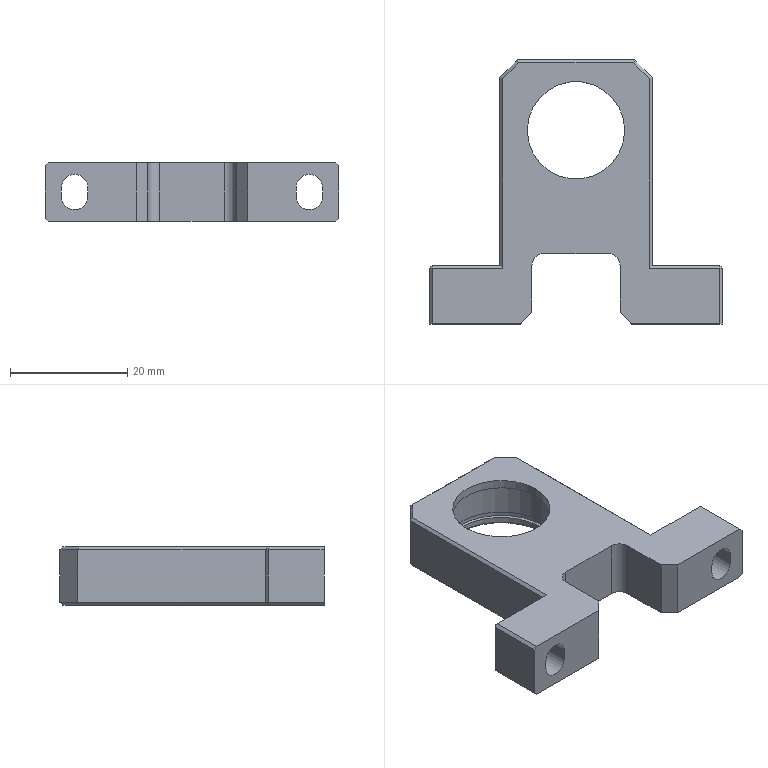Part | NX | features BREP 1 | 1 solid | 67 faces | box 50 x 45 x 10 mm | volume 8913 mm3 | plane 49 | cylinder 16 | cone 2 | commonest cylinder face diameters 4.5 x6 19 x4 4 x2 16.6 x2 20.2 x2